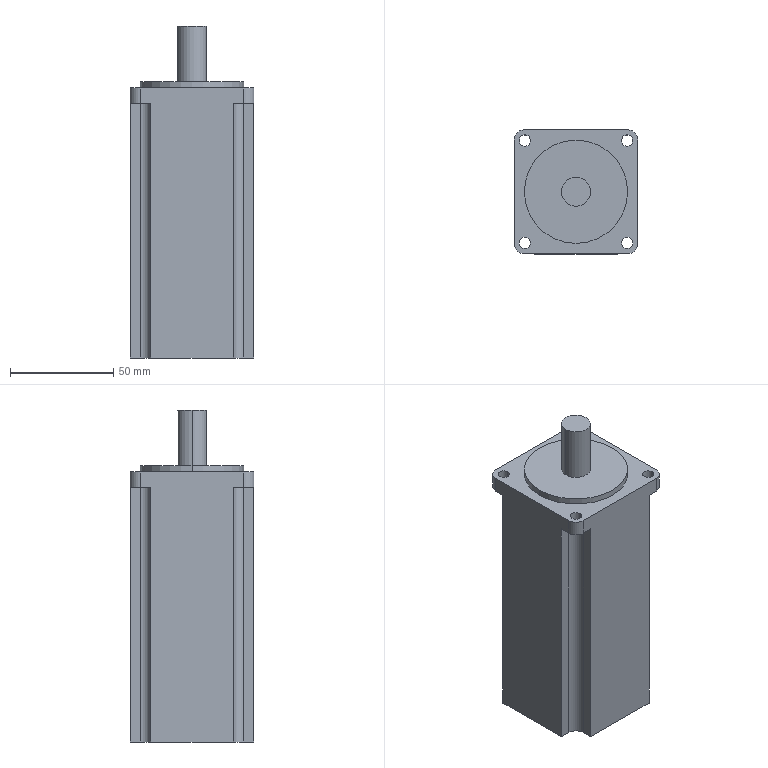Part | STEP file | SM140A-20-1140D-Delta motor 400W | 1 solid | 40 faces | box 60 x 60 x 160.7 mm | volume 433057 mm3 | cylinder 20 | plane 20 | commonest cylinder face diameters 5.5 x8 10 x8 14 x2 50 x2